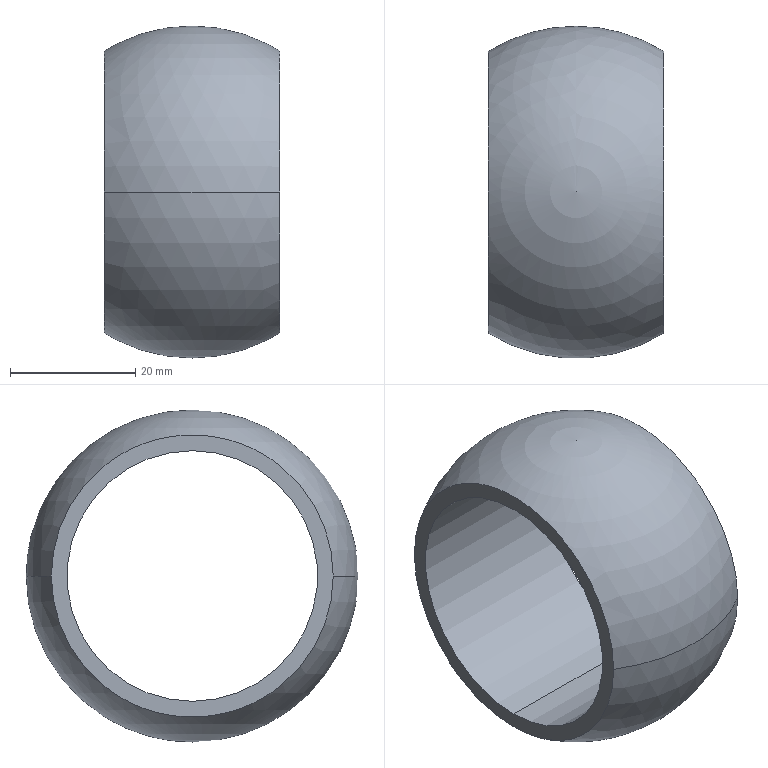Part | SolidWorks | features Revolution 1 | 1 solid | 6 faces | box 28 x 53 x 53 mm | volume 20840 mm3 | sphere 2 | cylinder 2 | plane 2 | commonest cylinder face diameters 40 x2
STEP:
#1=CARTESIAN_POINT('',(14.,22.5,0.));
#2=VERTEX_POINT('',#1);
#3=CARTESIAN_POINT('',(14.,-22.5,0.));
#4=VERTEX_POINT('',#3);
#5=CARTESIAN_POINT('',(14.,0.,0.));
#6=DIRECTION('',(-1.,0.,0.));
#7=DIRECTION('',(0.,0.,1.));
#8=AXIS2_PLACEMENT_3D('',#5,#6,#7);
#9=CIRCLE('',#8,22.5);
#10=EDGE_CURVE('',#2,#4,#9,.T.);
#11=ORIENTED_EDGE('',*,*,#10,.T.);
#12=CARTESIAN_POINT('',(-14.,-22.5,0.));
#13=VERTEX_POINT('',#12);
#14=CARTESIAN_POINT('',(0.,0.,0.));
#15=DIRECTION('',(0.,0.,-1.));
#16=DIRECTION('',(0.,1.,0.));
#17=AXIS2_PLACEMENT_3D('',#14,#15,#16);
#18=CIRCLE('',#17,26.5);
#19=EDGE_CURVE('',#4,#13,#18,.T.);
#20=ORIENTED_EDGE('',*,*,#19,.T.);
#21=CARTESIAN_POINT('',(-14.,22.5,0.));
#22=VERTEX_POINT('',#21);
#23=CARTESIAN_POINT('',(-14.,0.,0.));
#24=DIRECTION('',(-1.,0.,0.));
#25=DIRECTION('',(0.,0.,1.));
#26=AXIS2_PLACEMENT_3D('',#23,#24,#25);
#27=CIRCLE('',#26,22.5);
#28=EDGE_CURVE('',#22,#13,#27,.T.);
#29=ORIENTED_EDGE('',*,*,#28,.F.);
#30=CARTESIAN_POINT('',(0.,0.,0.));
#31=DIRECTION('',(0.,0.,1.));
#32=DIRECTION('',(1.,0.,0.));
#33=AXIS2_PLACEMENT_3D('',#30,#31,#32);
#34=CIRCLE('',#33,26.5);
#35=EDGE_CURVE('',#2,#22,#34,.T.);
#36=ORIENTED_EDGE('',*,*,#35,.F.);
#37=EDGE_LOOP('',(#11,#20,#29,#36));
#38=FACE_OUTER_BOUND('',#37,.T.);
#39=CARTESIAN_POINT('',(0.,0.,0.));
#40=DIRECTION('',(0.,0.,-1.));
#41=DIRECTION('',(0.,1.,0.));
#42=AXIS2_PLACEMENT_3D('',#39,#40,#41);
#43=SPHERICAL_SURFACE('',#42,26.5);
#44=ADVANCED_FACE('',(#38),#43,.T.);
#45=CARTESIAN_POINT('',(14.,0.,-20.));
#46=VERTEX_POINT('',#45);
#47=CARTESIAN_POINT('',(14.,0.,20.));
#48=VERTEX_POINT('',#47);
#49=CARTESIAN_POINT('',(14.,0.,0.));
#50=DIRECTION('',(-1.,0.,0.));
#51=DIRECTION('',(0.,0.,1.));
#52=AXIS2_PLACEMENT_3D('',#49,#50,#51);
#53=CIRCLE('',#52,20.);
#54=EDGE_CURVE('',#46,#48,#53,.T.);
#55=ORIENTED_EDGE('',*,*,#54,.F.);
#56=CARTESIAN_POINT('',(-14.,0.,-20.));
#57=VERTEX_POINT('',#56);
#58=CARTESIAN_POINT('',(-51.721,0.,-20.));
#59=DIRECTION('',(-1.,0.,0.));
#60=VECTOR('',#59,1000.);
#61=LINE('',#58,#60);
#62=EDGE_CURVE('',#46,#57,#61,.T.);
#63=ORIENTED_EDGE('',*,*,#62,.T.);
#64=CARTESIAN_POINT('',(-14.,0.,20.));
#65=VERTEX_POINT('',#64);
#66=CARTESIAN_POINT('',(-14.,0.,0.));
#67=DIRECTION('',(-1.,0.,0.));
#68=DIRECTION('',(0.,0.,1.));
#69=AXIS2_PLACEMENT_3D('',#66,#67,#68);
#70=CIRCLE('',#69,20.);
#71=EDGE_CURVE('',#57,#65,#70,.T.);
#72=ORIENTED_EDGE('',*,*,#71,.T.);
#73=CARTESIAN_POINT('',(-51.721,0.,20.));
#74=DIRECTION('',(-1.,0.,0.));
#75=VECTOR('',#74,1000.);
#76=LINE('',#73,#75);
#77=EDGE_CURVE('',#48,#65,#76,.T.);
#78=ORIENTED_EDGE('',*,*,#77,.F.);
#79=EDGE_LOOP('',(#55,#63,#72,#78));
#80=FACE_OUTER_BOUND('',#79,.T.);
#81=CARTESIAN_POINT('',(-51.721,0.,0.));
#82=DIRECTION('',(-1.,0.,0.));
#83=DIRECTION('',(0.,0.,1.));
#84=AXIS2_PLACEMENT_3D('',#81,#82,#83);
#85=CYLINDRICAL_SURFACE('',#84,20.);
#86=ADVANCED_FACE('',(#80),#85,.F.);
#87=ORIENTED_EDGE('',*,*,#62,.F.);
#88=CARTESIAN_POINT('',(14.,0.,0.));
#89=DIRECTION('',(-1.,0.,0.));
#90=DIRECTION('',(0.,0.,1.));
#91=AXIS2_PLACEMENT_3D('',#88,#89,#90);
#92=CIRCLE('',#91,20.);
#93=EDGE_CURVE('',#48,#46,#92,.T.);
#94=ORIENTED_EDGE('',*,*,#93,.F.);
#95=ORIENTED_EDGE('',*,*,#77,.T.);
#96=CARTESIAN_POINT('',(-14.,0.,0.));
#97=DIRECTION('',(-1.,0.,0.));
#98=DIRECTION('',(0.,0.,1.));
#99=AXIS2_PLACEMENT_3D('',#96,#97,#98);
#100=CIRCLE('',#99,20.);
#101=EDGE_CURVE('',#65,#57,#100,.T.);
#102=ORIENTED_EDGE('',*,*,#101,.T.);
#103=EDGE_LOOP('',(#87,#94,#95,#102));
#104=FACE_OUTER_BOUND('',#103,.T.);
#105=CARTESIAN_POINT('',(-51.721,0.,0.));
#106=DIRECTION('',(-1.,0.,0.));
#107=DIRECTION('',(0.,0.,1.));
#108=AXIS2_PLACEMENT_3D('',#105,#106,#107);
#109=CYLINDRICAL_SURFACE('',#108,20.);
#110=ADVANCED_FACE('',(#104),#109,.F.);
#111=ORIENTED_EDGE('',*,*,#10,.F.);
#112=CARTESIAN_POINT('',(14.,0.,0.));
#113=DIRECTION('',(-1.,0.,0.));
#114=DIRECTION('',(0.,0.,1.));
#115=AXIS2_PLACEMENT_3D('',#112,#113,#114);
#116=CIRCLE('',#115,22.5);
#117=EDGE_CURVE('',#4,#2,#116,.T.);
#118=ORIENTED_EDGE('',*,*,#117,.F.);
#119=EDGE_LOOP('',(#111,#118));
#120=FACE_OUTER_BOUND('',#119,.T.);
#121=ORIENTED_EDGE('',*,*,#93,.T.);
#122=ORIENTED_EDGE('',*,*,#54,.T.);
#123=EDGE_LOOP('',(#121,#122));
#124=FACE_BOUND('',#123,.T.);
#125=CARTESIAN_POINT('',(14.,22.5,0.));
#126=DIRECTION('',(-1.,0.,0.));
#127=DIRECTION('',(0.,0.,1.));
#128=AXIS2_PLACEMENT_3D('',#125,#126,#127);
#129=PLANE('',#128);
#130=ADVANCED_FACE('',(#120,#124),#129,.F.);
#131=ORIENTED_EDGE('',*,*,#19,.F.);
#132=ORIENTED_EDGE('',*,*,#117,.T.);
#133=ORIENTED_EDGE('',*,*,#35,.T.);
#134=CARTESIAN_POINT('',(-14.,0.,0.));
#135=DIRECTION('',(-1.,0.,0.));
#136=DIRECTION('',(0.,0.,1.));
#137=AXIS2_PLACEMENT_3D('',#134,#135,#136);
#138=CIRCLE('',#137,22.5);
#139=EDGE_CURVE('',#13,#22,#138,.T.);
#140=ORIENTED_EDGE('',*,*,#139,.F.);
#141=EDGE_LOOP('',(#131,#132,#133,#140));
#142=FACE_OUTER_BOUND('',#141,.T.);
#143=CARTESIAN_POINT('',(0.,0.,0.));
#144=DIRECTION('',(0.,0.,-1.));
#145=DIRECTION('',(0.,1.,0.));
#146=AXIS2_PLACEMENT_3D('',#143,#144,#145);
#147=SPHERICAL_SURFACE('',#146,26.5);
#148=ADVANCED_FACE('',(#142),#147,.T.);
#149=ORIENTED_EDGE('',*,*,#101,.F.);
#150=ORIENTED_EDGE('',*,*,#71,.F.);
#151=EDGE_LOOP('',(#149,#150));
#152=FACE_BOUND('',#151,.T.);
#153=ORIENTED_EDGE('',*,*,#28,.T.);
#154=ORIENTED_EDGE('',*,*,#139,.T.);
#155=EDGE_LOOP('',(#153,#154));
#156=FACE_OUTER_BOUND('',#155,.T.);
#157=CARTESIAN_POINT('',(-14.,22.5,0.));
#158=DIRECTION('',(1.,0.,0.));
#159=DIRECTION('',(0.,0.,-1.));
#160=AXIS2_PLACEMENT_3D('',#157,#158,#159);
#161=PLANE('',#160);
#162=ADVANCED_FACE('',(#152,#156),#161,.F.);
#163=CLOSED_SHELL('',(#44,#86,#110,#130,#148,#162));
#164=MANIFOLD_SOLID_BREP('',#163);
#165=CARTESIAN_POINT('',(0.,0.,0.));
#166=DIRECTION('',(0.,0.,1.));
#167=DIRECTION('',(1.,0.,0.));
#168=AXIS2_PLACEMENT_3D('',#165,#166,#167);
#169=(LENGTH_UNIT()NAMED_UNIT(*)SI_UNIT(.MILLI.,.METRE.));
#170=UNCERTAINTY_MEASURE_WITH_UNIT(LENGTH_MEASURE(0.00001),#169,'','');
#171=(NAMED_UNIT(*)PLANE_ANGLE_UNIT()SI_UNIT($,.RADIAN.));
#172=(NAMED_UNIT(*)SI_UNIT($,.STERADIAN.)SOLID_ANGLE_UNIT());
#173=(GEOMETRIC_REPRESENTATION_CONTEXT(3)GLOBAL_UNCERTAINTY_ASSIGNED_CONTEXT((#170))GLOBAL_UNIT_ASSIGNED_CONTEXT((#169,#171,#172))REPRESENTATION_CONTEXT('',''));
#174=ADVANCED_BREP_SHAPE_REPRESENTATION('',(#164,#168),#173);